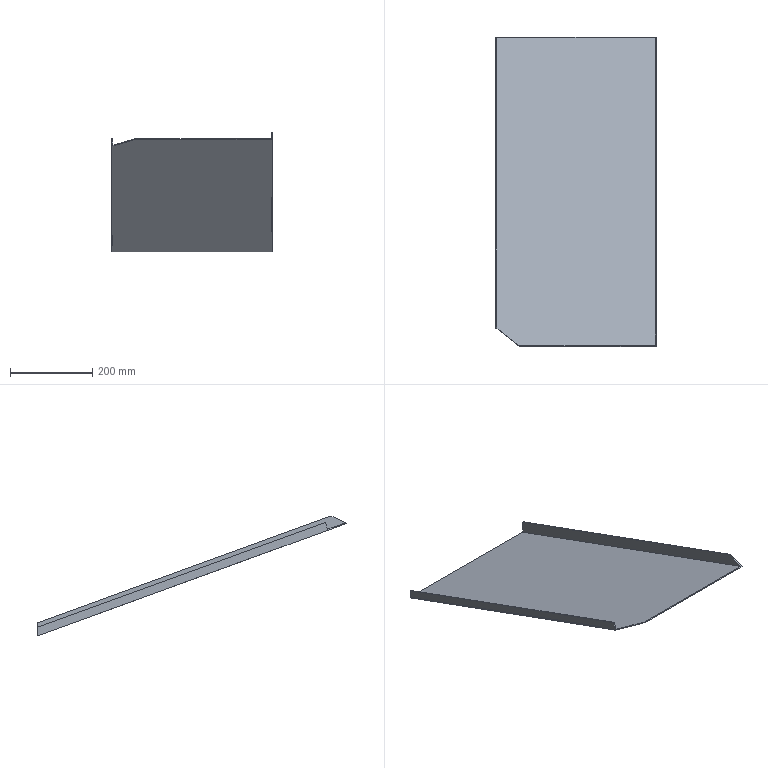Part | NX | features solid 2 | 1 solid | 12 faces | box 390 x 753.836 x 292.304 mm | volume 692670 mm3 | plane 11 | spline 1
STEP:
#1=CARTESIAN_POINT('',(580.,472.16,-120.897));
#2=VERTEX_POINT('',#1);
#3=CARTESIAN_POINT('',(635.864,428.727,-105.089));
#4=VERTEX_POINT('',#3);
#5=CARTESIAN_POINT('',(635.864,428.727,-105.089));
#6=CARTESIAN_POINT('',(617.243,443.205,-110.358));
#7=CARTESIAN_POINT('',(598.621,457.683,-115.628));
#8=CARTESIAN_POINT('',(580.,472.16,-120.897));
#9=B_SPLINE_CURVE_WITH_KNOTS('',3,(#5,#6,#7,#8),.UNSPECIFIED.,.F.,.F.,(4,4),(0.3656,0.4381),.UNSPECIFIED.);
#10=EDGE_CURVE('',#2,#4,#9,.F.);
#11=ORIENTED_EDGE('',*,*,#10,.T.);
#12=CARTESIAN_POINT('',(968.,428.727,-105.089));
#13=VERTEX_POINT('',#12);
#14=CARTESIAN_POINT('',(955.687,428.727,-105.089));
#15=DIRECTION('',(-1.,0.,0.));
#16=VECTOR('',#15,1000.);
#17=LINE('',#14,#16);
#18=EDGE_CURVE('',#4,#13,#17,.F.);
#19=ORIENTED_EDGE('',*,*,#18,.T.);
#20=CARTESIAN_POINT('',(968.,1180.,-378.53));
#21=VERTEX_POINT('',#20);
#22=CARTESIAN_POINT('',(968.,1053.844,-332.613));
#23=DIRECTION('',(0.,0.9397,-0.342));
#24=VECTOR('',#23,1000.);
#25=LINE('',#22,#24);
#26=EDGE_CURVE('',#13,#21,#25,.T.);
#27=ORIENTED_EDGE('',*,*,#26,.T.);
#28=CARTESIAN_POINT('',(582.,1180.,-378.53));
#29=VERTEX_POINT('',#28);
#30=CARTESIAN_POINT('',(920.,1180.,-378.53));
#31=DIRECTION('',(1.,0.,0.));
#32=VECTOR('',#31,1000.);
#33=LINE('',#30,#32);
#34=EDGE_CURVE('',#29,#21,#33,.T.);
#35=ORIENTED_EDGE('',*,*,#34,.F.);
#36=CARTESIAN_POINT('',(582.,472.16,-120.897));
#37=VERTEX_POINT('',#36);
#38=CARTESIAN_POINT('',(582.,1053.844,-332.613));
#39=DIRECTION('',(0.,-0.9397,0.342));
#40=VECTOR('',#39,1000.);
#41=LINE('',#38,#40);
#42=EDGE_CURVE('',#29,#37,#41,.T.);
#43=ORIENTED_EDGE('',*,*,#42,.T.);
#44=CARTESIAN_POINT('',(920.,472.16,-120.897));
#45=DIRECTION('',(-1.,0.,0.));
#46=VECTOR('',#45,1000.);
#47=LINE('',#44,#46);
#48=EDGE_CURVE('',#2,#37,#47,.F.);
#49=ORIENTED_EDGE('',*,*,#48,.F.);
#50=EDGE_LOOP('',(#11,#19,#27,#35,#43,#49));
#51=FACE_BOUND('',#50,.T.);
#52=CARTESIAN_POINT('',(920.,1053.844,-332.613));
#53=DIRECTION('',(0.,0.342,0.9397));
#54=DIRECTION('',(0.,-0.9397,0.342));
#55=AXIS2_PLACEMENT_3D('',#52,#53,#54);
#56=PLANE('',#55);
#57=ADVANCED_FACE('',(#51),#56,.T.);
#58=CARTESIAN_POINT('',(970.,464.615,-88.354));
#59=VERTEX_POINT('',#58);
#60=CARTESIAN_POINT('',(970.,426.164,-106.284));
#61=VERTEX_POINT('',#60);
#62=CARTESIAN_POINT('',(970.,406.483,-115.462));
#63=DIRECTION('',(0.,0.9063,0.4226));
#64=VECTOR('',#63,1000.);
#65=LINE('',#62,#64);
#66=EDGE_CURVE('',#59,#61,#65,.F.);
#67=ORIENTED_EDGE('',*,*,#66,.F.);
#68=CARTESIAN_POINT('',(968.,464.615,-88.354));
#69=VERTEX_POINT('',#68);
#70=CARTESIAN_POINT('',(880.,464.615,-88.354));
#71=DIRECTION('',(-1.,0.,0.));
#72=VECTOR('',#71,1000.);
#73=LINE('',#70,#72);
#74=EDGE_CURVE('',#69,#59,#73,.F.);
#75=ORIENTED_EDGE('',*,*,#74,.F.);
#76=CARTESIAN_POINT('',(968.,406.483,-115.462));
#77=DIRECTION('',(0.,-0.9063,-0.4226));
#78=VECTOR('',#77,1000.);
#79=LINE('',#76,#78);
#80=EDGE_CURVE('',#13,#69,#79,.F.);
#81=ORIENTED_EDGE('',*,*,#80,.F.);
#82=ORIENTED_EDGE('',*,*,#18,.F.);
#83=CARTESIAN_POINT('',(638.282,426.164,-106.284));
#84=VERTEX_POINT('',#83);
#85=CARTESIAN_POINT('',(638.282,426.164,-106.284));
#86=CARTESIAN_POINT('',(637.476,427.019,-105.886));
#87=CARTESIAN_POINT('',(636.67,427.873,-105.488));
#88=CARTESIAN_POINT('',(635.864,428.727,-105.089));
#89=B_SPLINE_CURVE_WITH_KNOTS('',3,(#85,#86,#87,#88),.UNSPECIFIED.,.F.,.F.,(4,4),(0.3774,0.3811),.UNSPECIFIED.);
#90=EDGE_CURVE('',#84,#4,#89,.T.);
#91=ORIENTED_EDGE('',*,*,#90,.F.);
#92=CARTESIAN_POINT('',(955.687,426.164,-106.284));
#93=DIRECTION('',(-1.,0.,0.));
#94=VECTOR('',#93,1000.);
#95=LINE('',#92,#94);
#96=EDGE_CURVE('',#84,#61,#95,.F.);
#97=ORIENTED_EDGE('',*,*,#96,.T.);
#98=EDGE_LOOP('',(#67,#75,#81,#82,#91,#97));
#99=FACE_BOUND('',#98,.T.);
#100=CARTESIAN_POINT('',(955.687,406.483,-115.462));
#101=DIRECTION('',(0.,0.4226,-0.9063));
#102=DIRECTION('',(0.,0.9063,0.4226));
#103=AXIS2_PLACEMENT_3D('',#100,#101,#102);
#104=PLANE('',#103);
#105=ADVANCED_FACE('',(#99),#104,.F.);
#106=CARTESIAN_POINT('',(968.,1180.,-348.733));
#107=VERTEX_POINT('',#106);
#108=CARTESIAN_POINT('',(968.,365.28,-52.199));
#109=DIRECTION('',(0.,0.9397,-0.342));
#110=VECTOR('',#109,1000.);
#111=LINE('',#108,#110);
#112=EDGE_CURVE('',#69,#107,#111,.T.);
#113=ORIENTED_EDGE('',*,*,#112,.T.);
#114=CARTESIAN_POINT('',(968.,1180.,-730.));
#115=DIRECTION('',(0.,0.,1.));
#116=VECTOR('',#115,1000.);
#117=LINE('',#114,#116);
#118=EDGE_CURVE('',#21,#107,#117,.T.);
#119=ORIENTED_EDGE('',*,*,#118,.F.);
#120=ORIENTED_EDGE('',*,*,#26,.F.);
#121=ORIENTED_EDGE('',*,*,#80,.T.);
#122=EDGE_LOOP('',(#113,#119,#120,#121));
#123=FACE_BOUND('',#122,.T.);
#124=CARTESIAN_POINT('',(968.,361.86,-61.596));
#125=DIRECTION('',(1.,0.,0.));
#126=DIRECTION('',(0.,0.,-1.));
#127=AXIS2_PLACEMENT_3D('',#124,#125,#126);
#128=PLANE('',#127);
#129=ADVANCED_FACE('',(#123),#128,.F.);
#130=CARTESIAN_POINT('',(970.,1180.,-348.733));
#131=VERTEX_POINT('',#130);
#132=CARTESIAN_POINT('',(970.,365.28,-52.199));
#133=DIRECTION('',(0.,0.9397,-0.342));
#134=VECTOR('',#133,1000.);
#135=LINE('',#132,#134);
#136=EDGE_CURVE('',#59,#131,#135,.T.);
#137=ORIENTED_EDGE('',*,*,#136,.T.);
#138=CARTESIAN_POINT('',(-675.,1180.,-348.733));
#139=DIRECTION('',(1.,0.,0.));
#140=VECTOR('',#139,1000.);
#141=LINE('',#138,#140);
#142=EDGE_CURVE('',#107,#131,#141,.T.);
#143=ORIENTED_EDGE('',*,*,#142,.F.);
#144=ORIENTED_EDGE('',*,*,#112,.F.);
#145=ORIENTED_EDGE('',*,*,#74,.T.);
#146=EDGE_LOOP('',(#137,#143,#144,#145));
#147=FACE_BOUND('',#146,.T.);
#148=CARTESIAN_POINT('',(880.,365.28,-52.199));
#149=DIRECTION('',(0.,-0.342,-0.9397));
#150=DIRECTION('',(0.,0.9397,-0.342));
#151=AXIS2_PLACEMENT_3D('',#148,#149,#150);
#152=PLANE('',#151);
#153=ADVANCED_FACE('',(#147),#152,.F.);
#154=CARTESIAN_POINT('',(970.,1180.,-380.658));
#155=VERTEX_POINT('',#154);
#156=CARTESIAN_POINT('',(970.,1053.16,-334.492));
#157=DIRECTION('',(0.,0.9397,-0.342));
#158=VECTOR('',#157,1000.);
#159=LINE('',#156,#158);
#160=EDGE_CURVE('',#61,#155,#159,.T.);
#161=ORIENTED_EDGE('',*,*,#160,.T.);
#162=CARTESIAN_POINT('',(970.,1180.,-313.819));
#163=DIRECTION('',(0.,0.,1.));
#164=VECTOR('',#163,1000.);
#165=LINE('',#162,#164);
#166=EDGE_CURVE('',#155,#131,#165,.T.);
#167=ORIENTED_EDGE('',*,*,#166,.T.);
#168=ORIENTED_EDGE('',*,*,#136,.F.);
#169=ORIENTED_EDGE('',*,*,#66,.T.);
#170=EDGE_LOOP('',(#161,#167,#168,#169));
#171=FACE_BOUND('',#170,.T.);
#172=CARTESIAN_POINT('',(970.,1060.684,-313.819));
#173=DIRECTION('',(-1.,0.,0.));
#174=DIRECTION('',(0.,0.,1.));
#175=AXIS2_PLACEMENT_3D('',#172,#173,#174);
#176=PLANE('',#175);
#177=ADVANCED_FACE('',(#171),#176,.F.);
#178=CARTESIAN_POINT('',(580.,471.476,-122.777));
#179=VERTEX_POINT('',#178);
#180=CARTESIAN_POINT('',(638.282,426.164,-106.284));
#181=CARTESIAN_POINT('',(618.854,441.268,-111.782));
#182=CARTESIAN_POINT('',(599.427,456.372,-117.279));
#183=CARTESIAN_POINT('',(580.,471.476,-122.777));
#184=B_SPLINE_CURVE_WITH_KNOTS('',3,(#180,#181,#182,#183),.UNSPECIFIED.,.F.,.F.,(4,4),(1.654,1.73),.UNSPECIFIED.);
#185=EDGE_CURVE('',#179,#84,#184,.F.);
#186=ORIENTED_EDGE('',*,*,#185,.T.);
#187=ORIENTED_EDGE('',*,*,#90,.T.);
#188=ORIENTED_EDGE('',*,*,#10,.F.);
#189=CARTESIAN_POINT('',(580.,471.818,-121.837));
#190=DIRECTION('',(0.,-0.342,-0.9397));
#191=VECTOR('',#190,1000.);
#192=LINE('',#189,#191);
#193=EDGE_CURVE('',#179,#2,#192,.F.);
#194=ORIENTED_EDGE('',*,*,#193,.F.);
#195=EDGE_LOOP('',(#186,#187,#188,#194));
#196=FACE_BOUND('',#195,.T.);
#197=CARTESIAN_POINT('',(580.,472.16,-120.897));
#198=CARTESIAN_POINT('',(580.,471.476,-122.777));
#199=CARTESIAN_POINT('',(594.462,460.916,-116.805));
#200=CARTESIAN_POINT('',(594.462,460.232,-118.684));
#201=CARTESIAN_POINT('',(608.924,449.673,-112.712));
#202=CARTESIAN_POINT('',(608.924,448.989,-114.592));
#203=CARTESIAN_POINT('',(623.778,438.124,-108.509));
#204=CARTESIAN_POINT('',(623.778,437.44,-110.389));
#205=CARTESIAN_POINT('',(638.631,426.576,-104.306));
#206=CARTESIAN_POINT('',(638.631,425.892,-106.185));
#207=B_SPLINE_SURFACE_WITH_KNOTS('',2,1,((#197,#198),(#199,#200),(#201,#202),(#203,#204),(#205,#206)),.SURF_OF_LINEAR_EXTRUSION.,.F.,.F.,.F.,(3,2,3),(2,2),(1.627,1.824,2.027),(0.,1.),.PIECEWISE_BEZIER_KNOTS.);
#208=ADVANCED_FACE('',(#196),#207,.F.);
#209=CARTESIAN_POINT('',(580.,1180.,-380.658));
#210=VERTEX_POINT('',#209);
#211=CARTESIAN_POINT('',(580.,1053.16,-334.492));
#212=DIRECTION('',(0.,-0.9397,0.342));
#213=VECTOR('',#212,1000.);
#214=LINE('',#211,#213);
#215=EDGE_CURVE('',#210,#179,#214,.T.);
#216=ORIENTED_EDGE('',*,*,#215,.F.);
#217=CARTESIAN_POINT('',(920.,1180.,-380.658));
#218=DIRECTION('',(1.,0.,0.));
#219=VECTOR('',#218,1000.);
#220=LINE('',#217,#219);
#221=EDGE_CURVE('',#210,#155,#220,.T.);
#222=ORIENTED_EDGE('',*,*,#221,.T.);
#223=ORIENTED_EDGE('',*,*,#160,.F.);
#224=ORIENTED_EDGE('',*,*,#96,.F.);
#225=ORIENTED_EDGE('',*,*,#185,.F.);
#226=EDGE_LOOP('',(#216,#222,#223,#224,#225));
#227=FACE_BOUND('',#226,.T.);
#228=CARTESIAN_POINT('',(920.,1053.16,-334.492));
#229=DIRECTION('',(0.,0.342,0.9397));
#230=DIRECTION('',(0.,-0.9397,0.342));
#231=AXIS2_PLACEMENT_3D('',#228,#229,#230);
#232=PLANE('',#231);
#233=ADVANCED_FACE('',(#227),#232,.F.);
#234=ORIENTED_EDGE('',*,*,#215,.T.);
#235=ORIENTED_EDGE('',*,*,#193,.T.);
#236=CARTESIAN_POINT('',(580.,478.316,-103.983));
#237=VERTEX_POINT('',#236);
#238=CARTESIAN_POINT('',(580.,471.476,-122.777));
#239=DIRECTION('',(0.,0.342,0.9397));
#240=VECTOR('',#239,1000.);
#241=LINE('',#238,#240);
#242=EDGE_CURVE('',#2,#237,#241,.T.);
#243=ORIENTED_EDGE('',*,*,#242,.T.);
#244=CARTESIAN_POINT('',(580.,1180.,-359.375));
#245=VERTEX_POINT('',#244);
#246=CARTESIAN_POINT('',(580.,1111.84,-334.567));
#247=DIRECTION('',(0.,-0.9397,0.342));
#248=VECTOR('',#247,1000.);
#249=LINE('',#246,#248);
#250=EDGE_CURVE('',#245,#237,#249,.T.);
#251=ORIENTED_EDGE('',*,*,#250,.F.);
#252=CARTESIAN_POINT('',(580.,1180.,-730.));
#253=DIRECTION('',(0.,0.,1.));
#254=VECTOR('',#253,1000.);
#255=LINE('',#252,#254);
#256=EDGE_CURVE('',#210,#245,#255,.T.);
#257=ORIENTED_EDGE('',*,*,#256,.F.);
#258=EDGE_LOOP('',(#234,#235,#243,#251,#257));
#259=FACE_BOUND('',#258,.T.);
#260=CARTESIAN_POINT('',(580.,985.,-145.));
#261=DIRECTION('',(1.,0.,0.));
#262=DIRECTION('',(0.,0.,1.));
#263=AXIS2_PLACEMENT_3D('',#260,#261,#262);
#264=PLANE('',#263);
#265=ADVANCED_FACE('',(#259),#264,.F.);
#266=ORIENTED_EDGE('',*,*,#221,.F.);
#267=ORIENTED_EDGE('',*,*,#256,.T.);
#268=CARTESIAN_POINT('',(582.,1180.,-359.375));
#269=VERTEX_POINT('',#268);
#270=CARTESIAN_POINT('',(-675.,1180.,-359.375));
#271=DIRECTION('',(1.,0.,0.));
#272=VECTOR('',#271,1000.);
#273=LINE('',#270,#272);
#274=EDGE_CURVE('',#245,#269,#273,.T.);
#275=ORIENTED_EDGE('',*,*,#274,.T.);
#276=CARTESIAN_POINT('',(582.,1180.,-730.));
#277=DIRECTION('',(0.,0.,1.));
#278=VECTOR('',#277,1000.);
#279=LINE('',#276,#278);
#280=EDGE_CURVE('',#29,#269,#279,.T.);
#281=ORIENTED_EDGE('',*,*,#280,.F.);
#282=ORIENTED_EDGE('',*,*,#34,.T.);
#283=ORIENTED_EDGE('',*,*,#118,.T.);
#284=ORIENTED_EDGE('',*,*,#142,.T.);
#285=ORIENTED_EDGE('',*,*,#166,.F.);
#286=EDGE_LOOP('',(#266,#267,#275,#281,#282,#283,#284,#285));
#287=FACE_BOUND('',#286,.T.);
#288=CARTESIAN_POINT('',(-675.,1180.,-730.));
#289=DIRECTION('',(0.,-1.,0.));
#290=DIRECTION('',(1.,0.,0.));
#291=AXIS2_PLACEMENT_3D('',#288,#289,#290);
#292=PLANE('',#291);
#293=ADVANCED_FACE('',(#287),#292,.F.);
#294=ORIENTED_EDGE('',*,*,#274,.F.);
#295=ORIENTED_EDGE('',*,*,#250,.T.);
#296=CARTESIAN_POINT('',(582.,478.316,-103.983));
#297=VERTEX_POINT('',#296);
#298=CARTESIAN_POINT('',(580.,478.316,-103.983));
#299=DIRECTION('',(-1.,0.,0.));
#300=VECTOR('',#299,1000.);
#301=LINE('',#298,#300);
#302=EDGE_CURVE('',#237,#297,#301,.F.);
#303=ORIENTED_EDGE('',*,*,#302,.T.);
#304=CARTESIAN_POINT('',(582.,1111.84,-334.567));
#305=DIRECTION('',(0.,-0.9397,0.342));
#306=VECTOR('',#305,1000.);
#307=LINE('',#304,#306);
#308=EDGE_CURVE('',#269,#297,#307,.T.);
#309=ORIENTED_EDGE('',*,*,#308,.F.);
#310=EDGE_LOOP('',(#294,#295,#303,#309));
#311=FACE_BOUND('',#310,.T.);
#312=CARTESIAN_POINT('',(580.,1111.84,-334.567));
#313=DIRECTION('',(0.,-0.342,-0.9397));
#314=DIRECTION('',(0.,-0.9397,0.342));
#315=AXIS2_PLACEMENT_3D('',#312,#313,#314);
#316=PLANE('',#315);
#317=ADVANCED_FACE('',(#311),#316,.F.);
#318=ORIENTED_EDGE('',*,*,#48,.T.);
#319=CARTESIAN_POINT('',(582.,471.476,-122.777));
#320=DIRECTION('',(0.,0.342,0.9397));
#321=VECTOR('',#320,1000.);
#322=LINE('',#319,#321);
#323=EDGE_CURVE('',#37,#297,#322,.T.);
#324=ORIENTED_EDGE('',*,*,#323,.T.);
#325=ORIENTED_EDGE('',*,*,#302,.F.);
#326=ORIENTED_EDGE('',*,*,#242,.F.);
#327=EDGE_LOOP('',(#318,#324,#325,#326));
#328=FACE_BOUND('',#327,.T.);
#329=CARTESIAN_POINT('',(580.,471.476,-122.777));
#330=DIRECTION('',(0.,-0.9397,0.342));
#331=DIRECTION('',(0.,0.342,0.9397));
#332=AXIS2_PLACEMENT_3D('',#329,#330,#331);
#333=PLANE('',#332);
#334=ADVANCED_FACE('',(#328),#333,.T.);
#335=ORIENTED_EDGE('',*,*,#42,.F.);
#336=ORIENTED_EDGE('',*,*,#280,.T.);
#337=ORIENTED_EDGE('',*,*,#308,.T.);
#338=ORIENTED_EDGE('',*,*,#323,.F.);
#339=EDGE_LOOP('',(#335,#336,#337,#338));
#340=FACE_BOUND('',#339,.T.);
#341=CARTESIAN_POINT('',(582.,1105.,-353.36));
#342=DIRECTION('',(1.,0.,0.));
#343=DIRECTION('',(0.,0.,1.));
#344=AXIS2_PLACEMENT_3D('',#341,#342,#343);
#345=PLANE('',#344);
#346=ADVANCED_FACE('',(#340),#345,.T.);
#347=CLOSED_SHELL('',(#57,#105,#129,#153,#177,#208,#233,#265,#293,#317,#334,#346));
#348=MANIFOLD_SOLID_BREP('',#347);
#349=(LENGTH_UNIT()NAMED_UNIT(*)SI_UNIT(.MILLI.,.METRE.));
#350=UNCERTAINTY_MEASURE_WITH_UNIT(LENGTH_MEASURE(0.0508),#349,'','');
#351=(NAMED_UNIT(*)PLANE_ANGLE_UNIT()SI_UNIT($,.RADIAN.));
#352=(NAMED_UNIT(*)SI_UNIT($,.STERADIAN.)SOLID_ANGLE_UNIT());
#353=(GEOMETRIC_REPRESENTATION_CONTEXT(3)GLOBAL_UNCERTAINTY_ASSIGNED_CONTEXT((#350))GLOBAL_UNIT_ASSIGNED_CONTEXT((#349,#351,#352))REPRESENTATION_CONTEXT('',''));
#354=ADVANCED_BREP_SHAPE_REPRESENTATION('',(#348),#353);